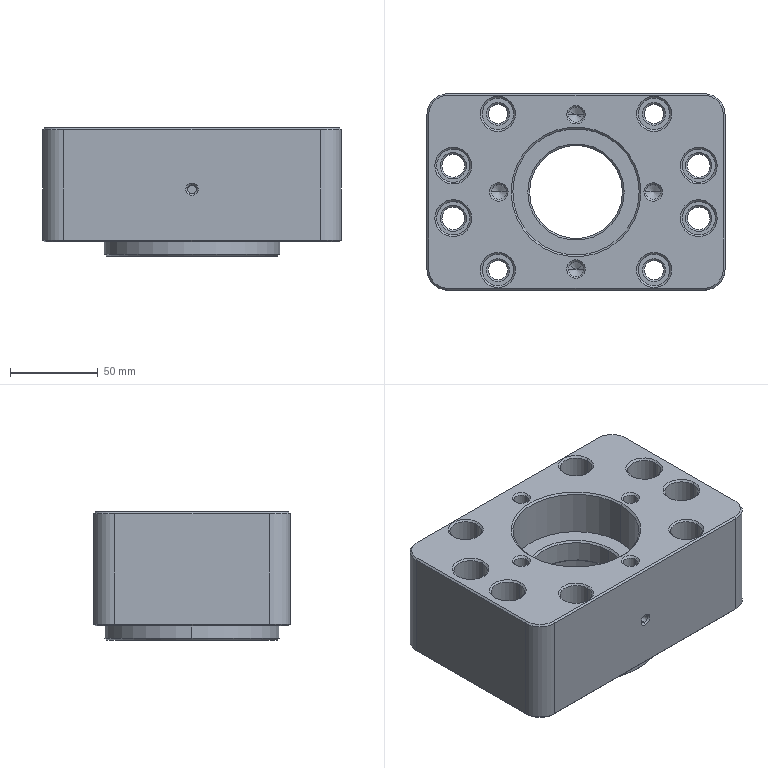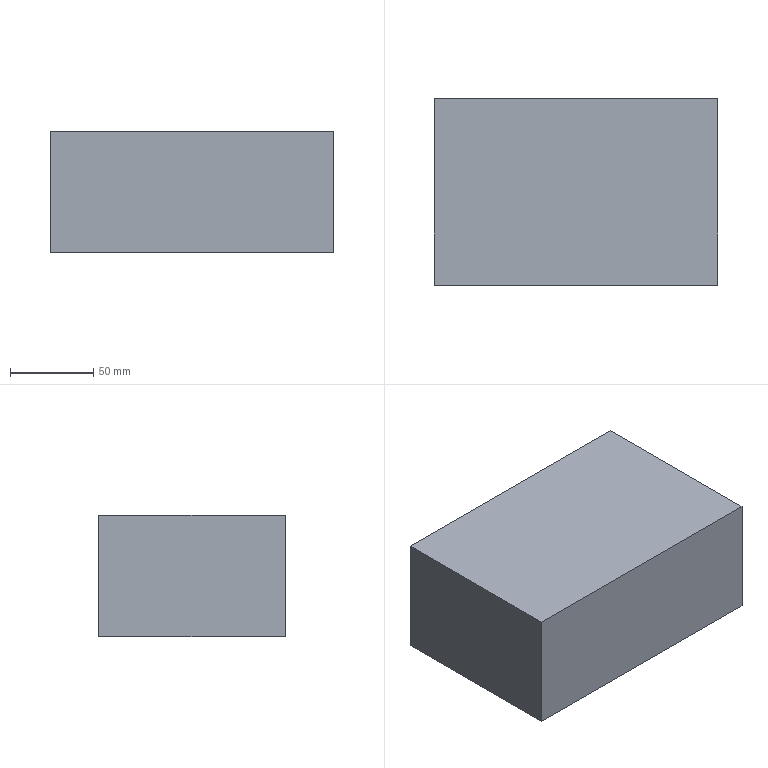CAM job | NX | 3-axis milling, drilling | part box 170 x 112 x 73 mm | stock box 170 x 112 x 73 mm
Tools:
number,name,description,diameter,corner_radius,flute_length,length,flutes
1,ZXZ,Milling Tool-5 Parameters,6.0,0.0,50.0,75.0,2
18,8.5ZT,Drilling Tool,8.5,0.0,35.0,50.0,2
14,13.0ZT,Drilling Tool,13.0,0.0,35.0,50.0,2
11,11.0ZT,Drilling Tool,11.0,0.0,35.0,50.0,2
10,D10C,Milling Tool-5 Parameters,10.0,0.0,50.0,75.0,2
9,D10JING,Milling Tool-5 Parameters,10.0,0.0,50.0,75.0,2
16,D26,Milling Tool-5 Parameters,26.0,0.0,50.0,75.0,2
7,D6A45,Milling Tool-5 Parameters,6.0,0.0,50.0,75.0,2
13,3.3ZT,Drilling Tool,3.3,0.0,35.0,50.0,2
5,D3R0.5,Milling Tool-5 Parameters,3.0,0.5,50.0,75.0,2
Operations:
program,operation,operation_type,tool,method,geometry_group,spindle_rpm,surface_speed,feed_per_tooth,feed_cut,feed_plunge,cut_length_mm,path_length_mm,cut_time_min,machine_time_min
1,DRILLING,Operation,ZXZ,METHOD,A,5000.0,94.0,0.025,250.0,0.0,52.0,654.512,0.208,0.2683
1,DRILLING_COPY_COPY_1,Operation,8.5ZT,METHOD,A,1573.0,42.0,0.0795,250.0,0.0,124.215,504.322,0.4969,0.5349
1,DRILLING_COPY_COPY_1_COPY,Operation,13.0ZT,METHOD,A,700.0,28.0,0.1071,150.0,0.0,343.028,961.659,2.287,2.349
1,DRILLING_COPY_COPY,Operation,11.0ZT,METHOD,A,1200.0,41.0,0.0625,150.0,0.0,291.219,918.59,1.942,2.004
1,HOLE_MILLING,CylinderMilling,D10C,METHOD,A,3500.0,109.0,0.3571,2500.0,1000.0,38150.56,39246.269,15.292,15.402
1,HOLE_MILLING_COPY,CylinderMilling,D10C,METHOD,A,3500.0,109.0,0.3571,2500.0,1000.0,80960.889,81157.389,32.472,32.491
1,HOLE_MILLING_COPY_COPY,CylinderMilling,D10C,METHOD,A,3500.0,109.0,0.3571,2500.0,1000.0,24875.22,25046.22,10.001,10.018
1,HOLE_MILLING_COPY_1,CylinderMilling,D10JING,METHOD,A,5000.0,157.0,0.12,1200.0,1000.0,4116.026,5211.734,3.438,3.548
1,HOLE_MILLING_COPY_1_COPY,CylinderMilling,D10JING,METHOD,A,5000.0,157.0,0.12,1200.0,1000.0,1161.824,1289.324,0.9721,0.9849
1,ZLEVEL_PROFILE,ZLevelMilling,D26,METHOD,A,1700.0,138.0,0.5,1700.0,1000.0,38212.469,165891.519,23.773,36.541
1,PLANAR_MILL_1,PlanarMilling,D6A45,METHOD,A,7500.0,141.0,0.0833,1250.0,100.0,1394.366,2744.559,1.115,1.25
1,PLANAR_MILL_1_COPY,PlanarMilling,D6A45,METHOD,A,7500.0,141.0,0.0833,1250.0,100.0,169.572,281.172,0.1357,0.1468
1,PLANAR_MILL_1_COPY_COPY,PlanarMilling,D6A45,METHOD,A,7500.0,141.0,0.0833,1250.0,100.0,326.136,1652.11,0.2609,0.3935
1,刀补9,CylinderMilling,D10JING,METHOD,A,5000.0,157.0,0.12,1200.0,1000.0,1330.622,1417.122,1.114,1.123
2,DRILLING_COPY,Operation,ZXZ,METHOD,B,5000.0,94.0,0.025,250.0,0.0,16.0,246.205,0.064,0.087
2,DRILLING_COPY_COPY_1_COPY_1,Operation,3.3ZT,METHOD,B,2000.0,20.0,0.03,120.0,0.0,69.966,354.136,0.583,0.6115
2,FLOOR_WALL,VolumeBased25DMillingOperation,D10C,METHOD,B,3500.0,109.0,0.3571,2500.0,1000.0,99250.606,102221.906,39.83,40.127
2,CAVITY_MILL,CavityMilling,D10C,METHOD,B,3500.0,109.0,0.3571,2500.0,1000.0,110223.934,115696.062,47.289,47.837
2,FLOOR_WALL_1,VolumeBased25DMillingOperation,D10JING,METHOD,B,5000.0,157.0,0.125,1250.0,100.0,4116.045,4738.154,3.293,3.355
2,ZLEVEL_PROFILE_COPY,ZLevelMilling,D10JING,METHOD,B,5000.0,157.0,0.12,1200.0,1000.0,459.263,551.596,0.3833,0.3925
2,ZLEVEL_PROFILE_1_COPY,ZLevelMilling,D3R0.5,METHOD,B,7000.0,65.0,0.1786,2500.0,100.0,8589.133,8680.93,3.436,3.445
2,DRILLING_COPY_1_COPY,Operation,D6A45,METHOD,B,5000.0,94.0,0.025,250.0,0.0,22.6,259.405,0.0904,0.1141
2,PLANAR_MILL_1_COPY_COPY_1,PlanarMilling,D6A45,METHOD,B,7500.0,141.0,0.0833,1250.0,100.0,587.959,714.759,0.4704,0.483
2,PLANAR_MILL_1_COPY_COPY_1_COPY,PlanarMilling,D6A45,METHOD,B,7500.0,141.0,0.0833,1250.0,100.0,882.655,1869.692,0.7061,0.8048
2,刀补,VolumeBased25DMillingOperation,D10JING,METHOD,B,5000.0,157.0,0.125,1250.0,100.0,227.275,348.275,0.1818,0.1939
2,PLANAR_MILL_1_COPY_COPY_1_COPY_COPY,PlanarMilling,D6A45,METHOD,B,7500.0,141.0,0.0833,1250.0,100.0,169.572,291.172,0.1357,0.1478
2,刀补_COPY,VolumeBased25DMillingOperation,D10JING,METHOD,B,5000.0,157.0,0.125,1250.0,100.0,353.451,426.451,0.2828,0.2901